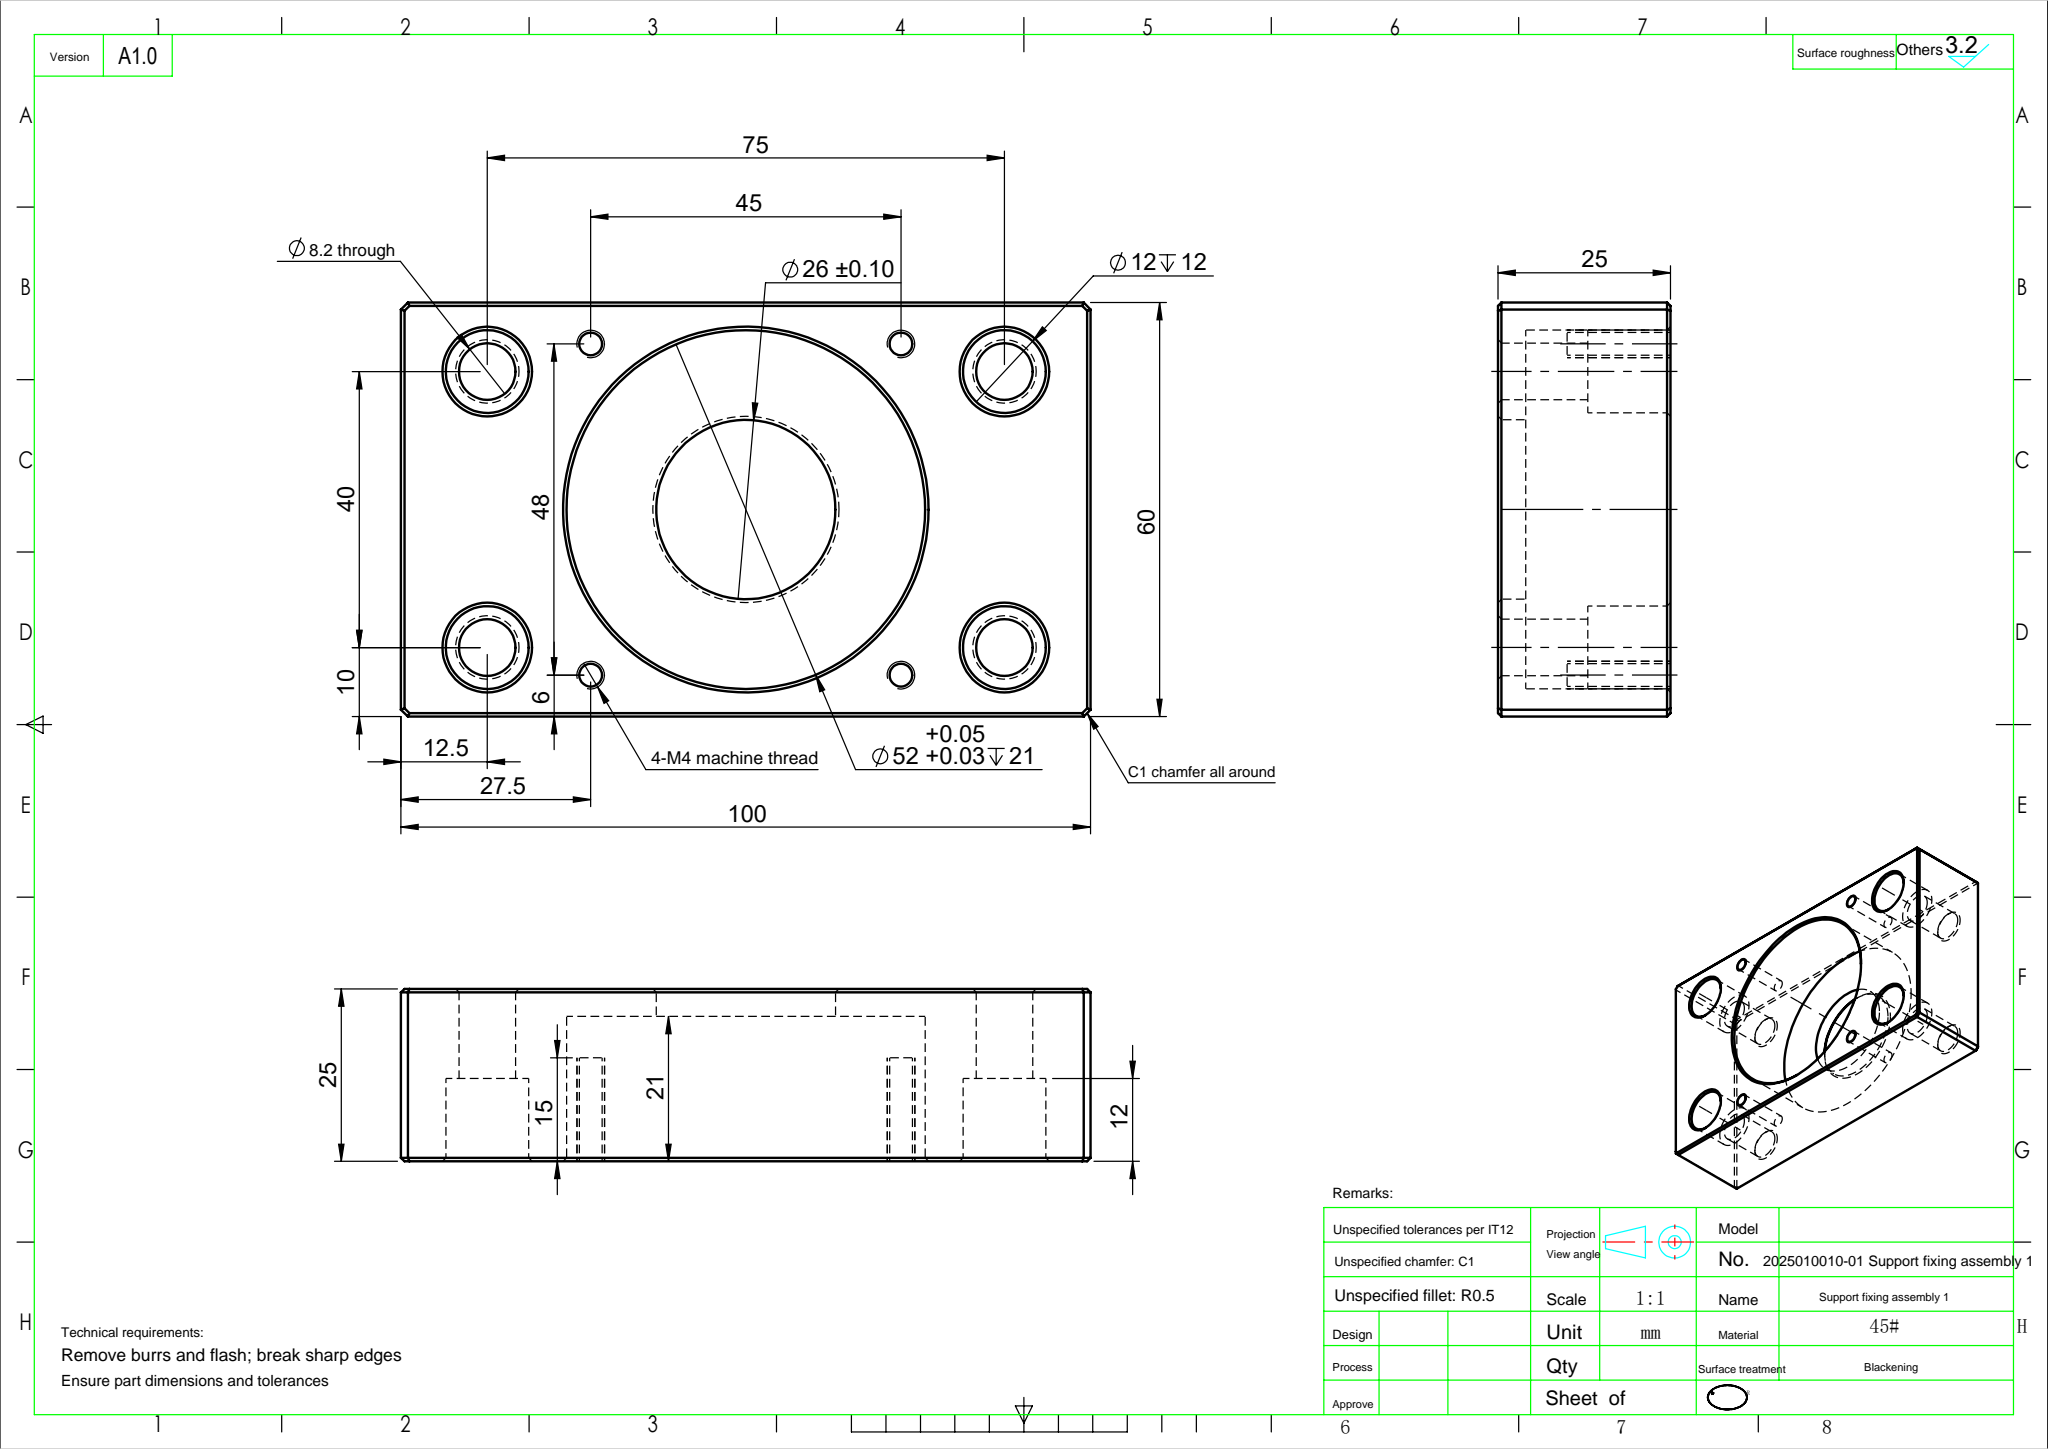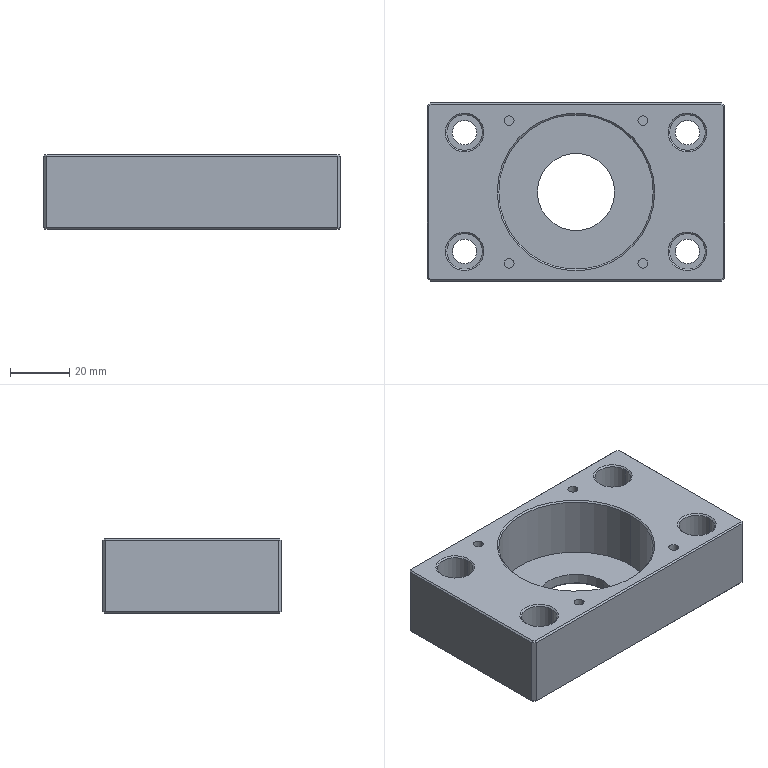Part | SolidWorks | features ICE 5, Chamfer 3, Extrusion 1 | 1 solid | 83 faces | box 100 x 60 x 25 mm | volume 94397 mm3 | plane 35 | cylinder 28 | cone 20 | commonest cylinder face diameters 3.3 x8 8.2 x8 12 x8 26 x2 52 x2